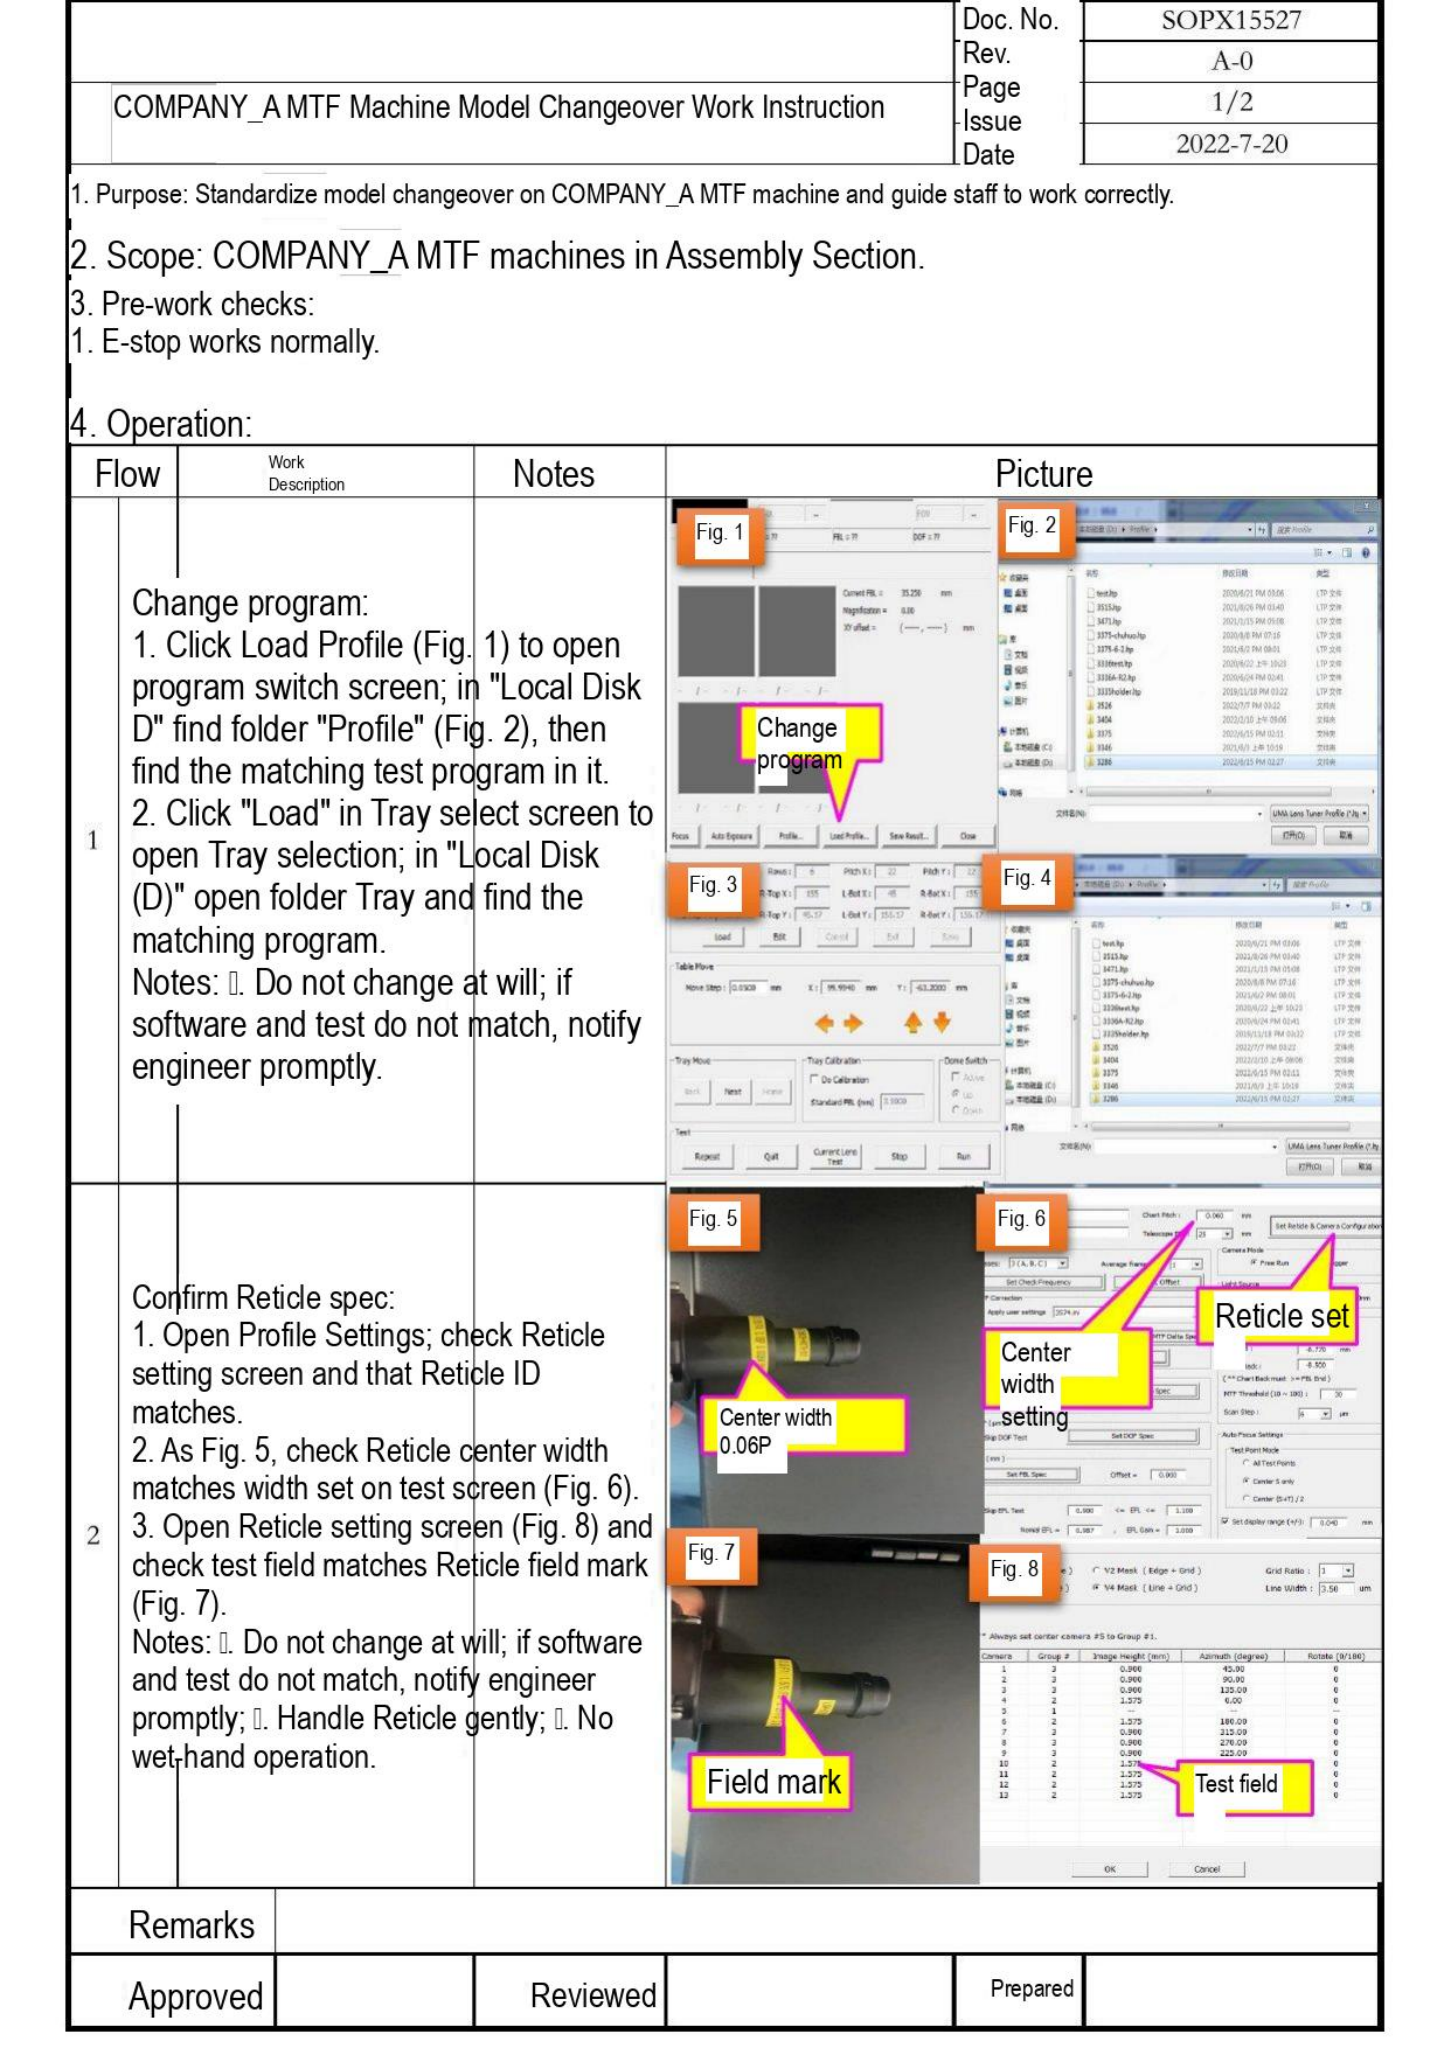| COMPANY_A MTF Machine Model Changeover Work Instruction | Doc. No. | SOPX15527 |
|---|---|---|
| | Rev. | A-0 |
| | Page | 1/2 |
| | Issue Date | 2022-7-20 |

1. Purpose: Standardize model changeover on COMPANY_A MTF machine and guide staff to work correctly.

2. Scope: COMPANY_A MTF machines in Assembly Section.

3. Pre-work checks:
1. E-stop works normally.

4. Operation:

| Flow | Work Description | Notes | Picture |
|---|---|---|---|
| 1 | Change program:<br>1. Click Load Profile (Fig. 1) to open program switch screen; in "Local Disk D" find folder "Profile" (Fig. 2), then find the matching test program in it.<br>2. Click "Load" in Tray select screen to open Tray selection; in "Local Disk (D)" open folder Tray and find the matching program.<br>Notes: ①. Do not change at will; if software and test do not match, notify engineer promptly. | | Fig. 1<br>Change program<br>Fig. 2<br>Fig. 3<br>Fig. 4 |
| 2 | Confirm Reticle spec:<br>1. Open Profile Settings; check Reticle setting screen and that Reticle ID matches.<br>2. As Fig. 5, check Reticle center width matches width set on test screen (Fig. 6).<br>3. Open Reticle setting screen (Fig. 8) and check test field matches Reticle field mark (Fig. 7).<br>Notes: ①. Do not change at will; if software and test do not match, notify engineer promptly; ②. Handle Reticle gently; ③. No wet-hand operation. | | Fig. 5<br>Center width 0.06P<br>Fig. 6<br>Center width setting<br>Reticle set<br>Fig. 7<br>Field mark<br>Fig. 8<br>Test field |

| Remarks | | | | | |
|---|---|---|---|---|---|
| Approved | | Reviewed | | Prepared | |
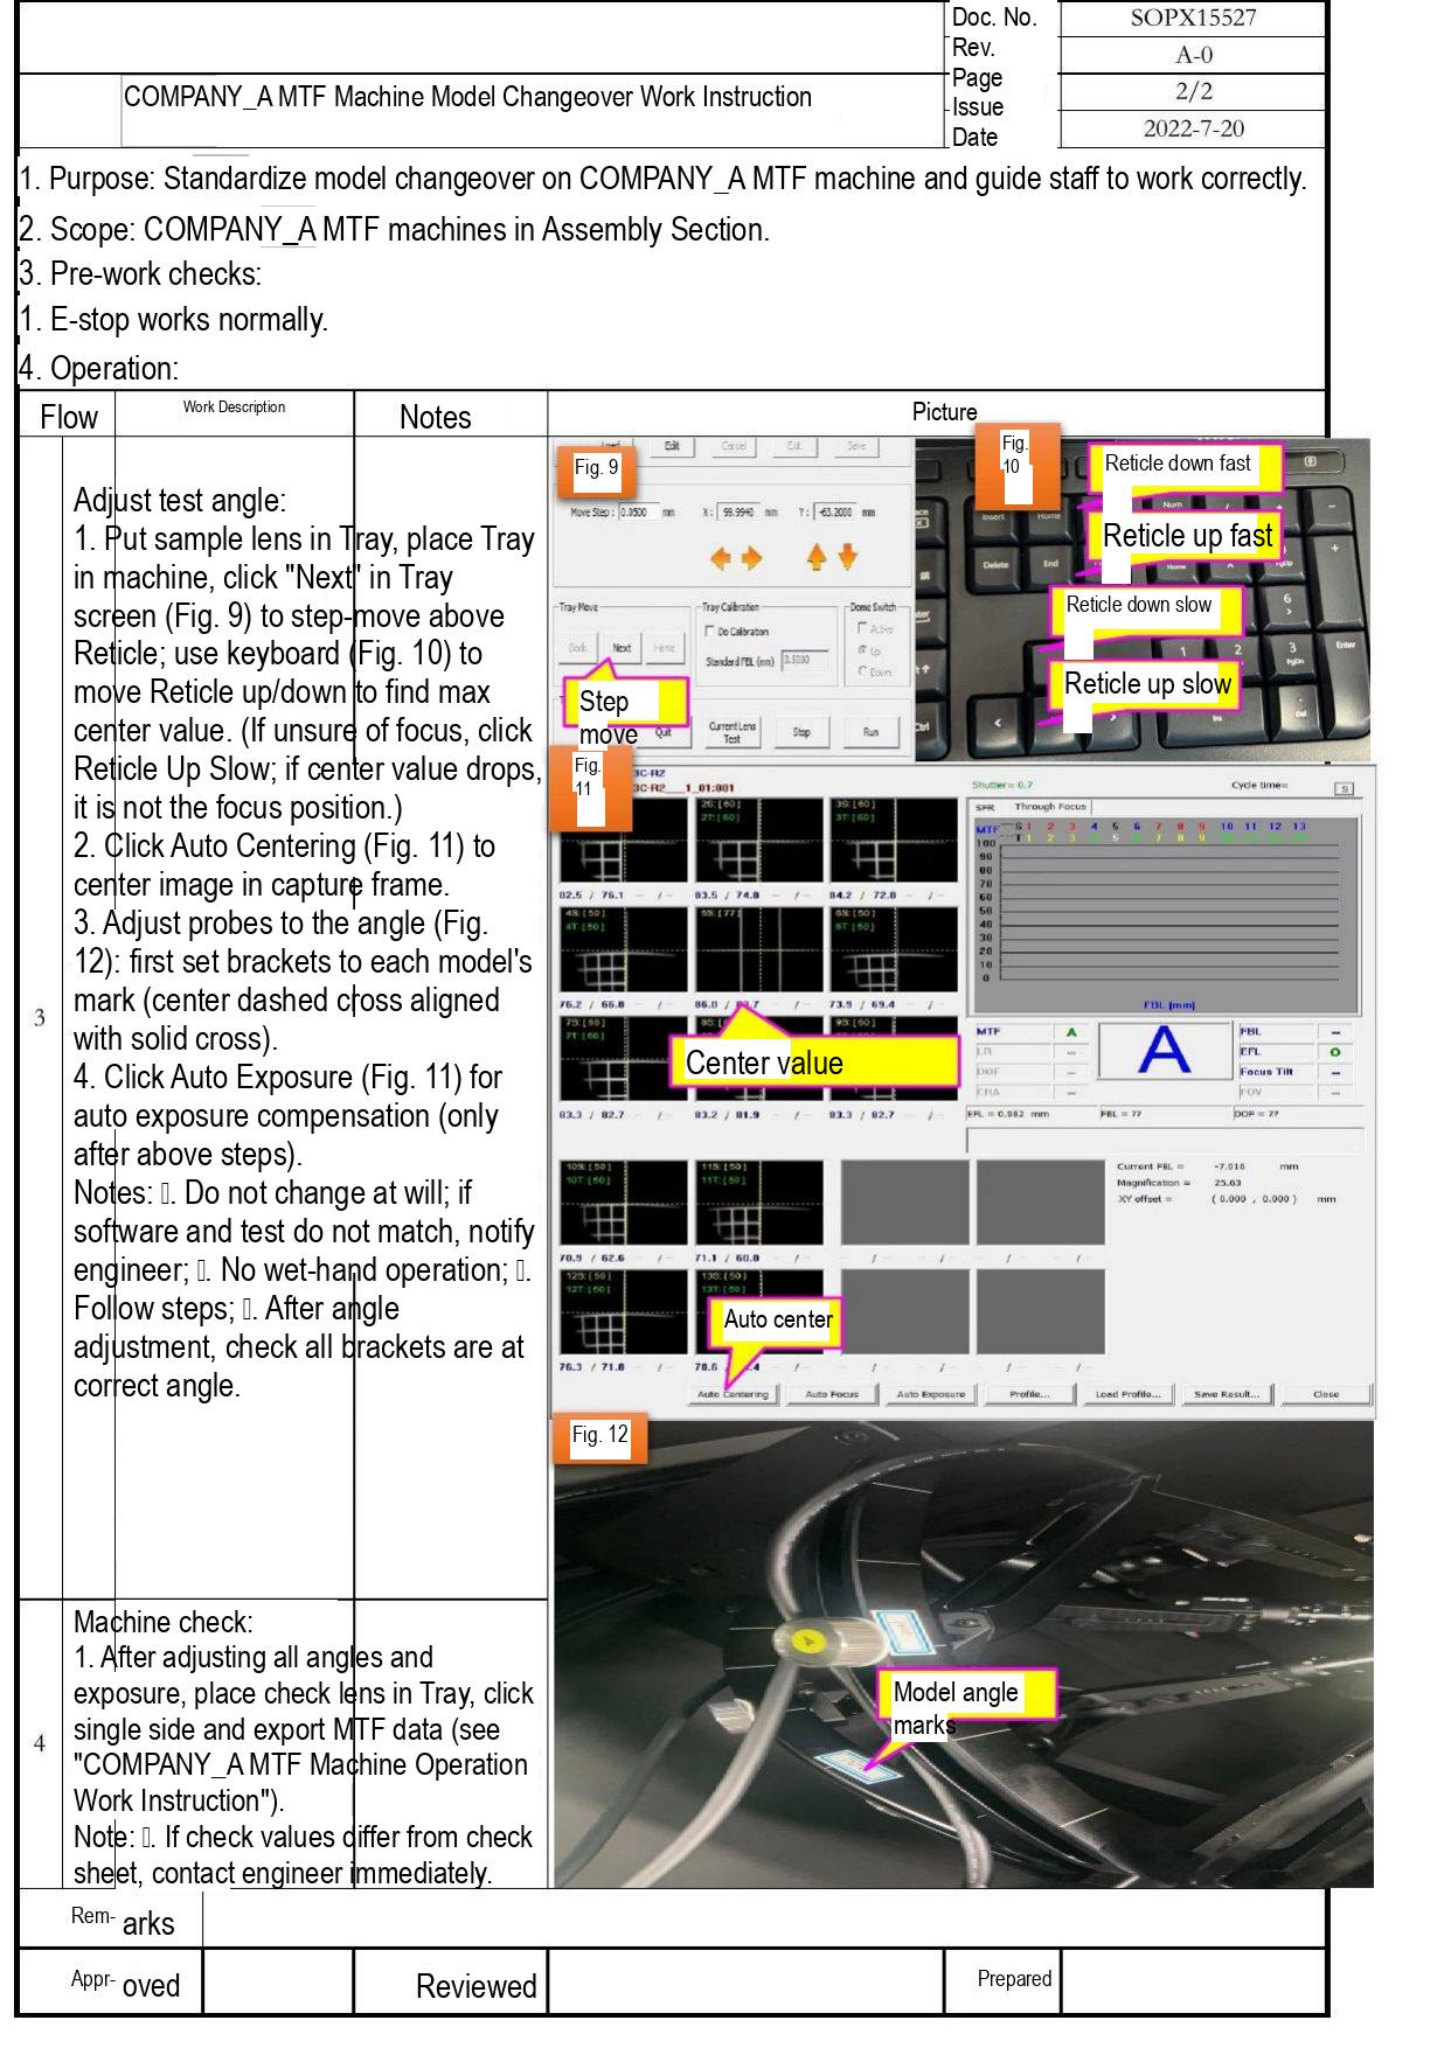| | Doc. No. | SOPX15527 |
|---|---|---|
| | Rev. | A-0 |
| COMPANY_A MTF Machine Model Changeover Work Instruction | Page | 2/2 |
| | Issue Date | 2022-7-20 |

1. Purpose: Standardize model changeover on COMPANY_A MTF machine and guide staff to work correctly.
2. Scope: COMPANY_A MTF machines in Assembly Section.
3. Pre-work checks:
1. E-stop works normally.
4. Operation:

| Flow | Work Description | Notes | Picture |
|---|---|---|---|
| 3 | Adjust test angle:<br>1. Put sample lens in Tray, place Tray in machine, click "Next" in Tray screen (Fig. 9) to step-move above Reticle; use keyboard (Fig. 10) to move Reticle up/down to find max center value. (If unsure of focus, click Reticle Up Slow; if center value drops, it is not the focus position.)<br>2. Click Auto Centering (Fig. 11) to center image in capture frame.<br>3. Adjust probes to the angle (Fig. 12): first set brackets to each model's mark (center dashed cross aligned with solid cross).<br>4. Click Auto Exposure (Fig. 11) for auto exposure compensation (only after above steps).<br>Notes: □. Do not change at will; if software and test do not match, notify engineer; □. No wet-hand operation; □. Follow steps; □. After angle adjustment, check all brackets are at correct angle. | | Fig. 9<br>Step move<br>Next<br>Stop<br>Run<br>Fig. 10<br>Reticle down fast<br>Reticle up fast<br>Reticle down slow<br>Reticle up slow<br>Fig. 11<br>Center value<br>Auto center<br>Auto Centering<br>Auto Focus<br>Auto Exposure<br>Profile...<br>Load Profile...<br>Save Result...<br>Close<br>Fig. 12 |
| 4 | Machine check:<br>1. After adjusting all angles and exposure, place check lens in Tray, click single side and export MTF data (see "COMPANY_A MTF Machine Operation Work Instruction").<br>Note: □. If check values differ from check sheet, contact engineer immediately. | | Model angle marks |

| Remarks | | | |
|---|---|---|---|
| Approved | | Reviewed | | Prepared | |